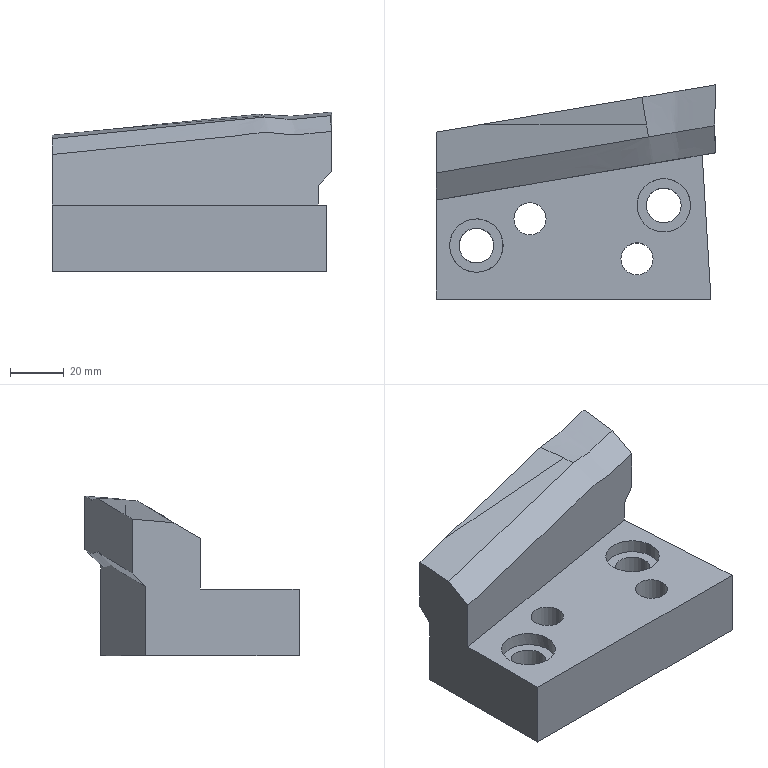Part | NX | features solid 2 | 1 solid | 24 faces | box 104.406 x 79.999 x 59.717 mm | volume 221865 mm3 | spline 10 | plane 8 | cylinder 6 | commonest cylinder face diameters 12 x2 13 x2 20 x2